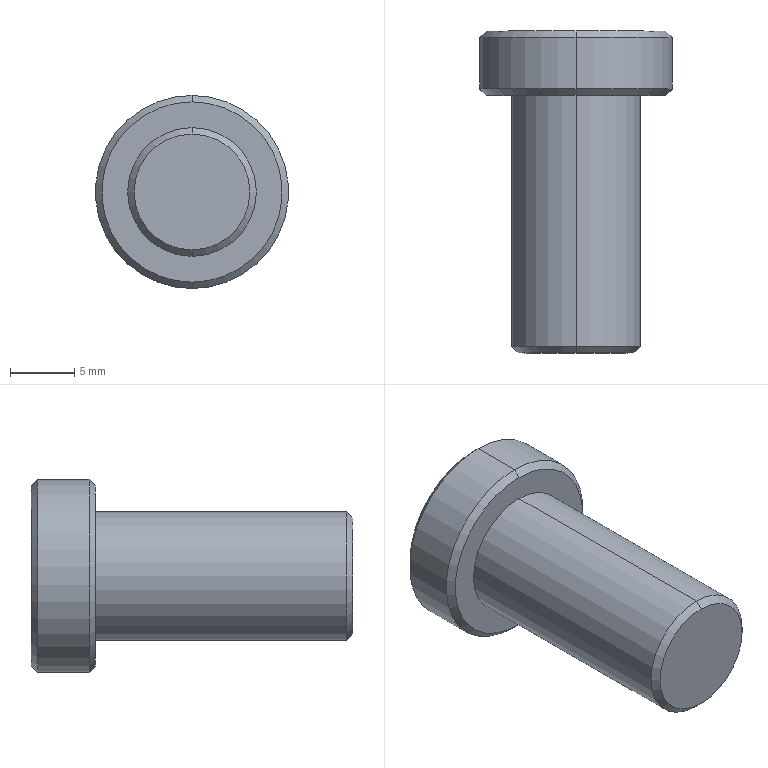Part | SolidWorks | features Chamfer 1, Extrusion 1, ICE 1 | 1 solid | 13 faces | box 15 x 25 x 15 mm | volume 2439 mm3 | cone 6 | cylinder 4 | plane 3 | commonest cylinder face diameters 10 x2 15 x2
STEP:
#1=CARTESIAN_POINT('',(0.,20.,-7.));
#2=VERTEX_POINT('',#1);
#3=CARTESIAN_POINT('',(0.,20.,7.));
#4=VERTEX_POINT('',#3);
#5=CARTESIAN_POINT('',(0.,20.,0.));
#6=DIRECTION('',(0.,-1.,0.));
#7=DIRECTION('',(0.,0.,1.));
#8=AXIS2_PLACEMENT_3D('',#5,#6,#7);
#9=CIRCLE('',#8,7.);
#10=EDGE_CURVE('',#2,#4,#9,.T.);
#11=ORIENTED_EDGE('',*,*,#10,.F.);
#12=CARTESIAN_POINT('',(0.,20.5,-7.5));
#13=VERTEX_POINT('',#12);
#14=CARTESIAN_POINT('',(0.,20.5,-7.5));
#15=DIRECTION('',(0.,0.7071,-0.7071));
#16=VECTOR('',#15,1000.);
#17=LINE('',#14,#16);
#18=EDGE_CURVE('',#2,#13,#17,.T.);
#19=ORIENTED_EDGE('',*,*,#18,.T.);
#20=CARTESIAN_POINT('',(0.,20.5,7.5));
#21=VERTEX_POINT('',#20);
#22=CARTESIAN_POINT('',(0.,20.5,0.));
#23=DIRECTION('',(0.,1.,0.));
#24=DIRECTION('',(0.,0.,1.));
#25=AXIS2_PLACEMENT_3D('',#22,#23,#24);
#26=CIRCLE('',#25,7.5);
#27=EDGE_CURVE('',#21,#13,#26,.T.);
#28=ORIENTED_EDGE('',*,*,#27,.F.);
#29=CARTESIAN_POINT('',(0.,20.5,7.5));
#30=DIRECTION('',(0.,0.7071,0.7071));
#31=VECTOR('',#30,1000.);
#32=LINE('',#29,#31);
#33=EDGE_CURVE('',#4,#21,#32,.T.);
#34=ORIENTED_EDGE('',*,*,#33,.F.);
#35=EDGE_LOOP('',(#11,#19,#28,#34));
#36=FACE_OUTER_BOUND('',#35,.T.);
#37=CARTESIAN_POINT('',(0.,20.5,0.));
#38=DIRECTION('',(0.,1.,0.));
#39=DIRECTION('',(0.,0.,1.));
#40=AXIS2_PLACEMENT_3D('',#37,#38,#39);
#41=CONICAL_SURFACE('',#40,7.5,0.7854);
#42=ADVANCED_FACE('',(#36),#41,.T.);
#43=CARTESIAN_POINT('',(0.,25.,7.));
#44=VERTEX_POINT('',#43);
#45=CARTESIAN_POINT('',(0.,25.,-7.));
#46=VERTEX_POINT('',#45);
#47=CARTESIAN_POINT('',(0.,25.,0.));
#48=DIRECTION('',(0.,1.,0.));
#49=DIRECTION('',(0.,0.,1.));
#50=AXIS2_PLACEMENT_3D('',#47,#48,#49);
#51=CIRCLE('',#50,7.);
#52=EDGE_CURVE('',#44,#46,#51,.T.);
#53=ORIENTED_EDGE('',*,*,#52,.F.);
#54=CARTESIAN_POINT('',(0.,24.5,7.5));
#55=VERTEX_POINT('',#54);
#56=CARTESIAN_POINT('',(0.,25.,7.));
#57=DIRECTION('',(0.,-0.7071,0.7071));
#58=VECTOR('',#57,1000.);
#59=LINE('',#56,#58);
#60=EDGE_CURVE('',#44,#55,#59,.T.);
#61=ORIENTED_EDGE('',*,*,#60,.T.);
#62=CARTESIAN_POINT('',(0.,24.5,-7.5));
#63=VERTEX_POINT('',#62);
#64=CARTESIAN_POINT('',(0.,24.5,0.));
#65=DIRECTION('',(0.,-1.,0.));
#66=DIRECTION('',(0.,0.,1.));
#67=AXIS2_PLACEMENT_3D('',#64,#65,#66);
#68=CIRCLE('',#67,7.5);
#69=EDGE_CURVE('',#63,#55,#68,.T.);
#70=ORIENTED_EDGE('',*,*,#69,.F.);
#71=CARTESIAN_POINT('',(0.,25.,-7.));
#72=DIRECTION('',(0.,-0.7071,-0.7071));
#73=VECTOR('',#72,1000.);
#74=LINE('',#71,#73);
#75=EDGE_CURVE('',#46,#63,#74,.T.);
#76=ORIENTED_EDGE('',*,*,#75,.F.);
#77=EDGE_LOOP('',(#53,#61,#70,#76));
#78=FACE_OUTER_BOUND('',#77,.T.);
#79=CARTESIAN_POINT('',(0.,25.,0.));
#80=DIRECTION('',(0.,-1.,0.));
#81=DIRECTION('',(0.,0.,-1.));
#82=AXIS2_PLACEMENT_3D('',#79,#80,#81);
#83=CONICAL_SURFACE('',#82,7.,0.7854);
#84=ADVANCED_FACE('',(#78),#83,.T.);
#85=CARTESIAN_POINT('',(0.,0.,-4.5));
#86=VERTEX_POINT('',#85);
#87=CARTESIAN_POINT('',(0.,0.,4.5));
#88=VERTEX_POINT('',#87);
#89=CARTESIAN_POINT('',(0.,0.,0.));
#90=DIRECTION('',(0.,-1.,0.));
#91=DIRECTION('',(0.,0.,1.));
#92=AXIS2_PLACEMENT_3D('',#89,#90,#91);
#93=CIRCLE('',#92,4.5);
#94=EDGE_CURVE('',#86,#88,#93,.T.);
#95=ORIENTED_EDGE('',*,*,#94,.F.);
#96=CARTESIAN_POINT('',(0.,0.5,-5.));
#97=VERTEX_POINT('',#96);
#98=CARTESIAN_POINT('',(0.,0.5,-5.));
#99=DIRECTION('',(0.,0.7071,-0.7071));
#100=VECTOR('',#99,1000.);
#101=LINE('',#98,#100);
#102=EDGE_CURVE('',#86,#97,#101,.T.);
#103=ORIENTED_EDGE('',*,*,#102,.T.);
#104=CARTESIAN_POINT('',(0.,0.5,5.));
#105=VERTEX_POINT('',#104);
#106=CARTESIAN_POINT('',(0.,0.5,0.));
#107=DIRECTION('',(0.,1.,0.));
#108=DIRECTION('',(0.,0.,1.));
#109=AXIS2_PLACEMENT_3D('',#106,#107,#108);
#110=CIRCLE('',#109,5.);
#111=EDGE_CURVE('',#105,#97,#110,.T.);
#112=ORIENTED_EDGE('',*,*,#111,.F.);
#113=CARTESIAN_POINT('',(0.,0.5,5.));
#114=DIRECTION('',(0.,0.7071,0.7071));
#115=VECTOR('',#114,1000.);
#116=LINE('',#113,#115);
#117=EDGE_CURVE('',#88,#105,#116,.T.);
#118=ORIENTED_EDGE('',*,*,#117,.F.);
#119=EDGE_LOOP('',(#95,#103,#112,#118));
#120=FACE_OUTER_BOUND('',#119,.T.);
#121=CARTESIAN_POINT('',(0.,0.5,0.));
#122=DIRECTION('',(0.,1.,0.));
#123=DIRECTION('',(0.,0.,1.));
#124=AXIS2_PLACEMENT_3D('',#121,#122,#123);
#125=CONICAL_SURFACE('',#124,5.,0.7854);
#126=ADVANCED_FACE('',(#120),#125,.T.);
#127=ORIENTED_EDGE('',*,*,#69,.T.);
#128=CARTESIAN_POINT('',(0.,25.,7.5));
#129=DIRECTION('',(0.,-1.,0.));
#130=VECTOR('',#129,1000.);
#131=LINE('',#128,#130);
#132=EDGE_CURVE('',#55,#21,#131,.T.);
#133=ORIENTED_EDGE('',*,*,#132,.T.);
#134=ORIENTED_EDGE('',*,*,#27,.T.);
#135=CARTESIAN_POINT('',(0.,25.,-7.5));
#136=DIRECTION('',(0.,-1.,0.));
#137=VECTOR('',#136,1000.);
#138=LINE('',#135,#137);
#139=EDGE_CURVE('',#63,#13,#138,.T.);
#140=ORIENTED_EDGE('',*,*,#139,.F.);
#141=EDGE_LOOP('',(#127,#133,#134,#140));
#142=FACE_OUTER_BOUND('',#141,.T.);
#143=CARTESIAN_POINT('',(0.,25.,0.));
#144=DIRECTION('',(0.,-1.,0.));
#145=DIRECTION('',(0.,0.,-1.));
#146=AXIS2_PLACEMENT_3D('',#143,#144,#145);
#147=CYLINDRICAL_SURFACE('',#146,7.5);
#148=ADVANCED_FACE('',(#142),#147,.T.);
#149=CARTESIAN_POINT('',(0.,20.,5.));
#150=VERTEX_POINT('',#149);
#151=CARTESIAN_POINT('',(0.,20.,-5.));
#152=VERTEX_POINT('',#151);
#153=CARTESIAN_POINT('',(0.,20.,0.));
#154=DIRECTION('',(0.,1.,0.));
#155=DIRECTION('',(0.,0.,1.));
#156=AXIS2_PLACEMENT_3D('',#153,#154,#155);
#157=CIRCLE('',#156,5.);
#158=EDGE_CURVE('',#150,#152,#157,.T.);
#159=ORIENTED_EDGE('',*,*,#158,.F.);
#160=CARTESIAN_POINT('',(0.,20.,5.));
#161=DIRECTION('',(0.,-1.,0.));
#162=VECTOR('',#161,1000.);
#163=LINE('',#160,#162);
#164=EDGE_CURVE('',#150,#105,#163,.T.);
#165=ORIENTED_EDGE('',*,*,#164,.T.);
#166=ORIENTED_EDGE('',*,*,#111,.T.);
#167=CARTESIAN_POINT('',(0.,20.,-5.));
#168=DIRECTION('',(0.,-1.,0.));
#169=VECTOR('',#168,1000.);
#170=LINE('',#167,#169);
#171=EDGE_CURVE('',#152,#97,#170,.T.);
#172=ORIENTED_EDGE('',*,*,#171,.F.);
#173=EDGE_LOOP('',(#159,#165,#166,#172));
#174=FACE_OUTER_BOUND('',#173,.T.);
#175=CARTESIAN_POINT('',(0.,20.,0.));
#176=DIRECTION('',(0.,-1.,0.));
#177=DIRECTION('',(0.,0.,-1.));
#178=AXIS2_PLACEMENT_3D('',#175,#176,#177);
#179=CYLINDRICAL_SURFACE('',#178,5.);
#180=ADVANCED_FACE('',(#174),#179,.T.);
#181=ORIENTED_EDGE('',*,*,#164,.F.);
#182=CARTESIAN_POINT('',(0.,20.,0.));
#183=DIRECTION('',(0.,1.,0.));
#184=DIRECTION('',(0.,0.,1.));
#185=AXIS2_PLACEMENT_3D('',#182,#183,#184);
#186=CIRCLE('',#185,5.);
#187=EDGE_CURVE('',#152,#150,#186,.T.);
#188=ORIENTED_EDGE('',*,*,#187,.F.);
#189=ORIENTED_EDGE('',*,*,#171,.T.);
#190=CARTESIAN_POINT('',(0.,0.5,0.));
#191=DIRECTION('',(0.,1.,0.));
#192=DIRECTION('',(0.,0.,1.));
#193=AXIS2_PLACEMENT_3D('',#190,#191,#192);
#194=CIRCLE('',#193,5.);
#195=EDGE_CURVE('',#97,#105,#194,.T.);
#196=ORIENTED_EDGE('',*,*,#195,.T.);
#197=EDGE_LOOP('',(#181,#188,#189,#196));
#198=FACE_OUTER_BOUND('',#197,.T.);
#199=CARTESIAN_POINT('',(0.,20.,0.));
#200=DIRECTION('',(0.,-1.,0.));
#201=DIRECTION('',(0.,0.,-1.));
#202=AXIS2_PLACEMENT_3D('',#199,#200,#201);
#203=CYLINDRICAL_SURFACE('',#202,5.);
#204=ADVANCED_FACE('',(#198),#203,.T.);
#205=CARTESIAN_POINT('',(0.,0.,0.));
#206=DIRECTION('',(0.,-1.,0.));
#207=DIRECTION('',(0.,0.,1.));
#208=AXIS2_PLACEMENT_3D('',#205,#206,#207);
#209=CIRCLE('',#208,4.5);
#210=EDGE_CURVE('',#88,#86,#209,.T.);
#211=ORIENTED_EDGE('',*,*,#210,.T.);
#212=ORIENTED_EDGE('',*,*,#94,.T.);
#213=EDGE_LOOP('',(#211,#212));
#214=FACE_OUTER_BOUND('',#213,.T.);
#215=CARTESIAN_POINT('',(0.,0.,0.));
#216=DIRECTION('',(0.,1.,0.));
#217=DIRECTION('',(0.,0.,1.));
#218=AXIS2_PLACEMENT_3D('',#215,#216,#217);
#219=PLANE('',#218);
#220=ADVANCED_FACE('',(#214),#219,.F.);
#221=ORIENTED_EDGE('',*,*,#132,.F.);
#222=CARTESIAN_POINT('',(0.,24.5,0.));
#223=DIRECTION('',(0.,-1.,0.));
#224=DIRECTION('',(0.,0.,1.));
#225=AXIS2_PLACEMENT_3D('',#222,#223,#224);
#226=CIRCLE('',#225,7.5);
#227=EDGE_CURVE('',#55,#63,#226,.T.);
#228=ORIENTED_EDGE('',*,*,#227,.T.);
#229=ORIENTED_EDGE('',*,*,#139,.T.);
#230=CARTESIAN_POINT('',(0.,20.5,0.));
#231=DIRECTION('',(0.,1.,0.));
#232=DIRECTION('',(0.,0.,1.));
#233=AXIS2_PLACEMENT_3D('',#230,#231,#232);
#234=CIRCLE('',#233,7.5);
#235=EDGE_CURVE('',#13,#21,#234,.T.);
#236=ORIENTED_EDGE('',*,*,#235,.T.);
#237=EDGE_LOOP('',(#221,#228,#229,#236));
#238=FACE_OUTER_BOUND('',#237,.T.);
#239=CARTESIAN_POINT('',(0.,25.,0.));
#240=DIRECTION('',(0.,-1.,0.));
#241=DIRECTION('',(0.,0.,-1.));
#242=AXIS2_PLACEMENT_3D('',#239,#240,#241);
#243=CYLINDRICAL_SURFACE('',#242,7.5);
#244=ADVANCED_FACE('',(#238),#243,.T.);
#245=CARTESIAN_POINT('',(0.,25.,0.));
#246=DIRECTION('',(0.,1.,0.));
#247=DIRECTION('',(0.,0.,1.));
#248=AXIS2_PLACEMENT_3D('',#245,#246,#247);
#249=CIRCLE('',#248,7.);
#250=EDGE_CURVE('',#46,#44,#249,.T.);
#251=ORIENTED_EDGE('',*,*,#250,.T.);
#252=ORIENTED_EDGE('',*,*,#52,.T.);
#253=EDGE_LOOP('',(#251,#252));
#254=FACE_OUTER_BOUND('',#253,.T.);
#255=CARTESIAN_POINT('',(0.,25.,0.));
#256=DIRECTION('',(0.,1.,0.));
#257=DIRECTION('',(0.,0.,1.));
#258=AXIS2_PLACEMENT_3D('',#255,#256,#257);
#259=PLANE('',#258);
#260=ADVANCED_FACE('',(#254),#259,.T.);
#261=CARTESIAN_POINT('',(0.,20.,0.));
#262=DIRECTION('',(0.,-1.,0.));
#263=DIRECTION('',(0.,0.,1.));
#264=AXIS2_PLACEMENT_3D('',#261,#262,#263);
#265=CIRCLE('',#264,7.);
#266=EDGE_CURVE('',#4,#2,#265,.T.);
#267=ORIENTED_EDGE('',*,*,#266,.T.);
#268=ORIENTED_EDGE('',*,*,#10,.T.);
#269=EDGE_LOOP('',(#267,#268));
#270=FACE_OUTER_BOUND('',#269,.T.);
#271=ORIENTED_EDGE('',*,*,#187,.T.);
#272=ORIENTED_EDGE('',*,*,#158,.T.);
#273=EDGE_LOOP('',(#271,#272));
#274=FACE_BOUND('',#273,.T.);
#275=CARTESIAN_POINT('',(0.,20.,0.));
#276=DIRECTION('',(0.,1.,0.));
#277=DIRECTION('',(0.,0.,1.));
#278=AXIS2_PLACEMENT_3D('',#275,#276,#277);
#279=PLANE('',#278);
#280=ADVANCED_FACE('',(#270,#274),#279,.F.);
#281=ORIENTED_EDGE('',*,*,#102,.F.);
#282=ORIENTED_EDGE('',*,*,#210,.F.);
#283=ORIENTED_EDGE('',*,*,#117,.T.);
#284=ORIENTED_EDGE('',*,*,#195,.F.);
#285=EDGE_LOOP('',(#281,#282,#283,#284));
#286=FACE_OUTER_BOUND('',#285,.T.);
#287=CARTESIAN_POINT('',(0.,0.5,0.));
#288=DIRECTION('',(0.,1.,0.));
#289=DIRECTION('',(0.,0.,1.));
#290=AXIS2_PLACEMENT_3D('',#287,#288,#289);
#291=CONICAL_SURFACE('',#290,5.,0.7854);
#292=ADVANCED_FACE('',(#286),#291,.T.);
#293=ORIENTED_EDGE('',*,*,#60,.F.);
#294=ORIENTED_EDGE('',*,*,#250,.F.);
#295=ORIENTED_EDGE('',*,*,#75,.T.);
#296=ORIENTED_EDGE('',*,*,#227,.F.);
#297=EDGE_LOOP('',(#293,#294,#295,#296));
#298=FACE_OUTER_BOUND('',#297,.T.);
#299=CARTESIAN_POINT('',(0.,25.,0.));
#300=DIRECTION('',(0.,-1.,0.));
#301=DIRECTION('',(0.,0.,-1.));
#302=AXIS2_PLACEMENT_3D('',#299,#300,#301);
#303=CONICAL_SURFACE('',#302,7.,0.7854);
#304=ADVANCED_FACE('',(#298),#303,.T.);
#305=ORIENTED_EDGE('',*,*,#18,.F.);
#306=ORIENTED_EDGE('',*,*,#266,.F.);
#307=ORIENTED_EDGE('',*,*,#33,.T.);
#308=ORIENTED_EDGE('',*,*,#235,.F.);
#309=EDGE_LOOP('',(#305,#306,#307,#308));
#310=FACE_OUTER_BOUND('',#309,.T.);
#311=CARTESIAN_POINT('',(0.,20.5,0.));
#312=DIRECTION('',(0.,1.,0.));
#313=DIRECTION('',(0.,0.,1.));
#314=AXIS2_PLACEMENT_3D('',#311,#312,#313);
#315=CONICAL_SURFACE('',#314,7.5,0.7854);
#316=ADVANCED_FACE('',(#310),#315,.T.);
#317=CLOSED_SHELL('',(#42,#84,#126,#148,#180,#204,#220,#244,#260,#280,#292,#304,#316));
#318=MANIFOLD_SOLID_BREP('',#317);
#319=CARTESIAN_POINT('',(0.,0.,0.));
#320=DIRECTION('',(0.,0.,1.));
#321=DIRECTION('',(1.,0.,0.));
#322=AXIS2_PLACEMENT_3D('',#319,#320,#321);
#323=(LENGTH_UNIT()NAMED_UNIT(*)SI_UNIT(.MILLI.,.METRE.));
#324=UNCERTAINTY_MEASURE_WITH_UNIT(LENGTH_MEASURE(0.00001),#323,'','');
#325=(NAMED_UNIT(*)PLANE_ANGLE_UNIT()SI_UNIT($,.RADIAN.));
#326=(NAMED_UNIT(*)SI_UNIT($,.STERADIAN.)SOLID_ANGLE_UNIT());
#327=(GEOMETRIC_REPRESENTATION_CONTEXT(3)GLOBAL_UNCERTAINTY_ASSIGNED_CONTEXT((#324))GLOBAL_UNIT_ASSIGNED_CONTEXT((#323,#325,#326))REPRESENTATION_CONTEXT('',''));
#328=ADVANCED_BREP_SHAPE_REPRESENTATION('',(#318,#322),#327);